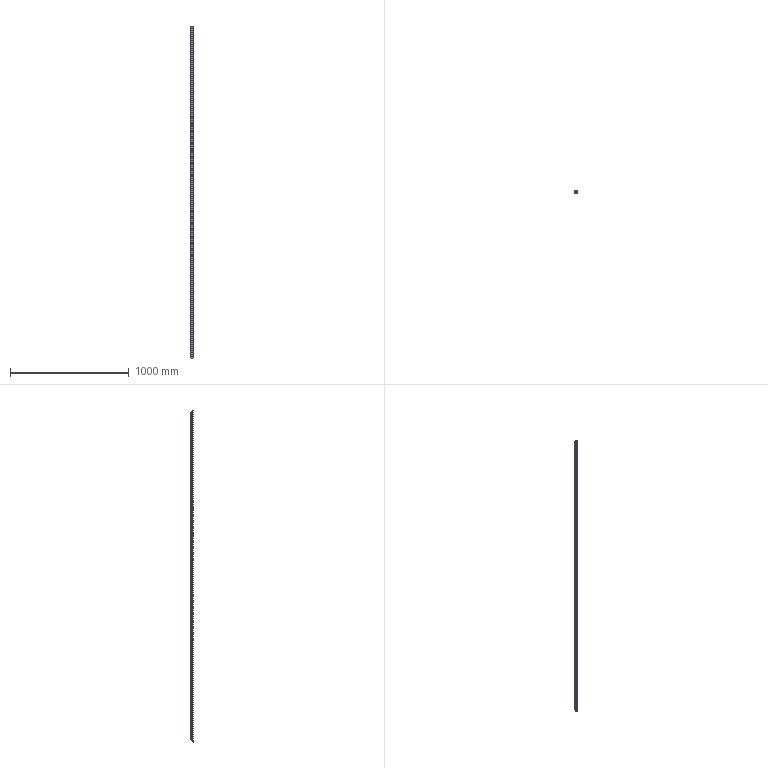Part | STEP file | DIN EN 10210-2 - 20 x 20 x 2 - 2500 | 1 solid | 18 faces | box 20 x 20 x 2800 mm | volume 388388 mm3 | plane 10 | cylinder 8 | commonest cylinder face diameters 4 x4 6 x4